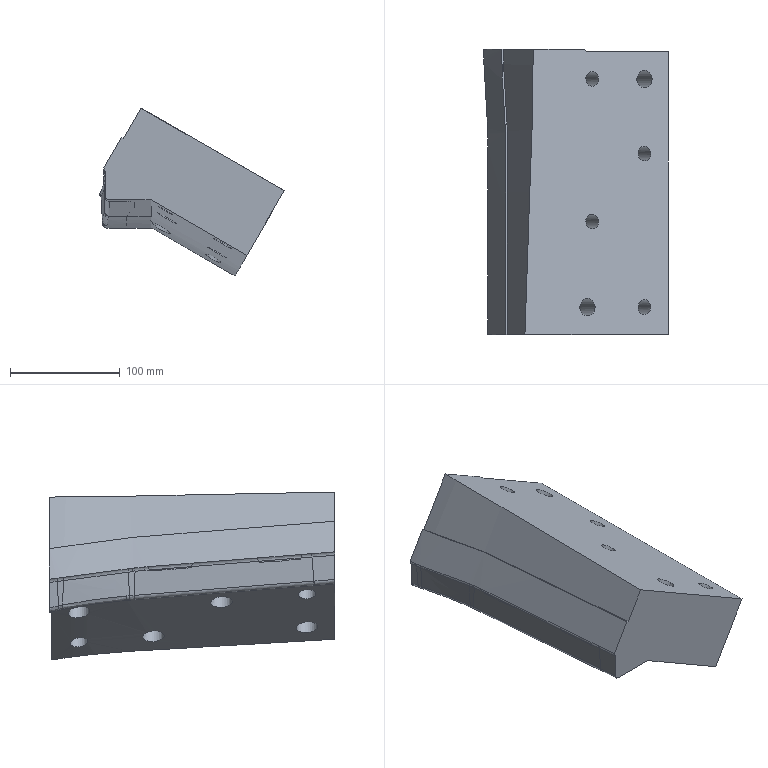Part | NX | features solid 2 | 1 solid | 55 faces | box 168.146 x 260 x 153.126 mm | volume 2952001 mm3 | spline 35 | plane 10 | cylinder 10 | commonest cylinder face diameters 13.5 x4 19.5 x4 16 x2